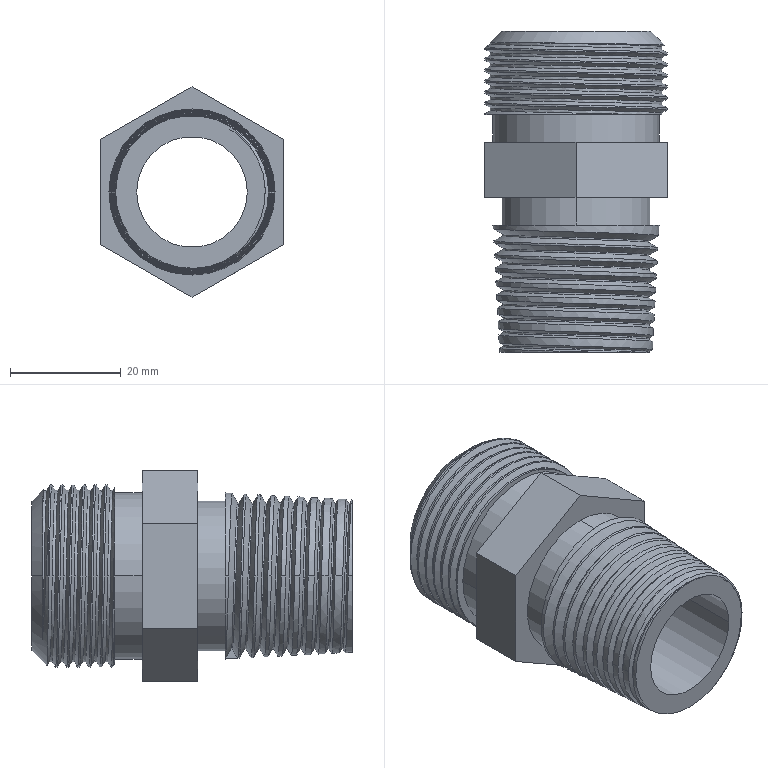Part | SolidWorks | features BaseBody 1 | 1 solid | 93 faces | box 33 x 58 x 38 mm | volume 23357 mm3 | cylinder 53 | cone 23 | plane 13 | spline 4 | commonest cylinder face diameters 26.5 x18 31 x15 33 x14 20 x2 27 x2 30 x2